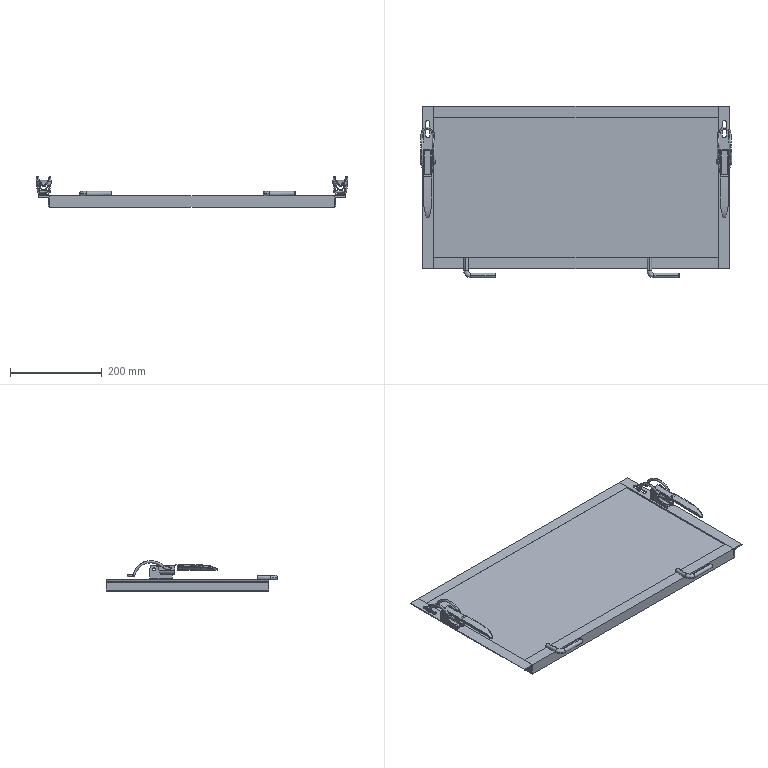Part | SolidWorks | 13 solids | 372 faces | box 679.336 x 374 x 67.182 mm | volume 1003039 mm3 | plane 162 | cylinder 114 | spline 76 | torus 16 | cone 4 | commonest cylinder face diameters 6 x48 8 x12 4 x10 204 x10 10 x8 18.5 x8